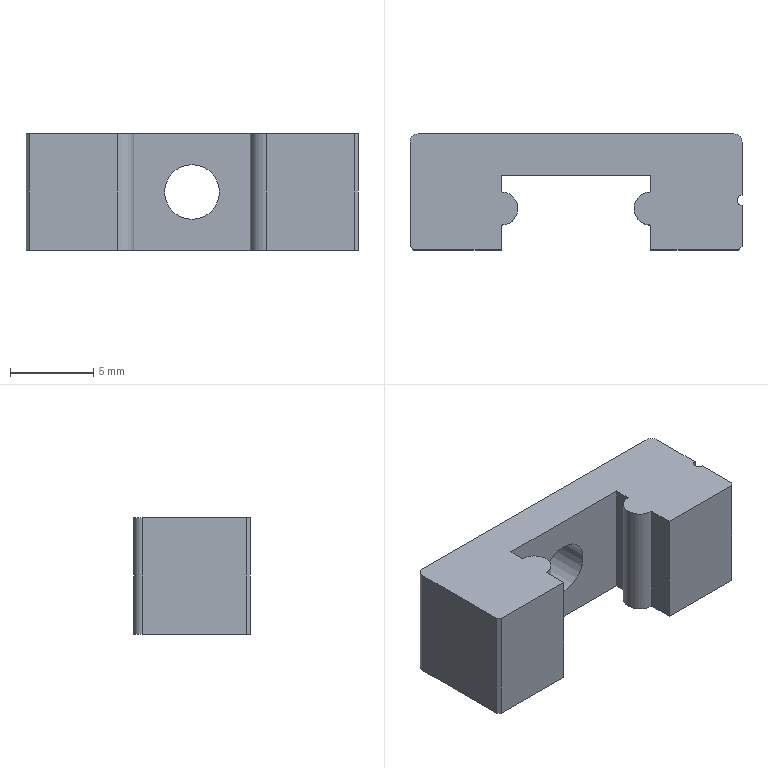Part | STEP file | MGN9 limit block 1001 | 1 solid | 24 faces | box 20 x 7 x 7 mm | volume 695.088 mm3 | plane 15 | cylinder 9 | commonest cylinder face diameters 2 x3 0.6 x2 1 x2 3.3 x2